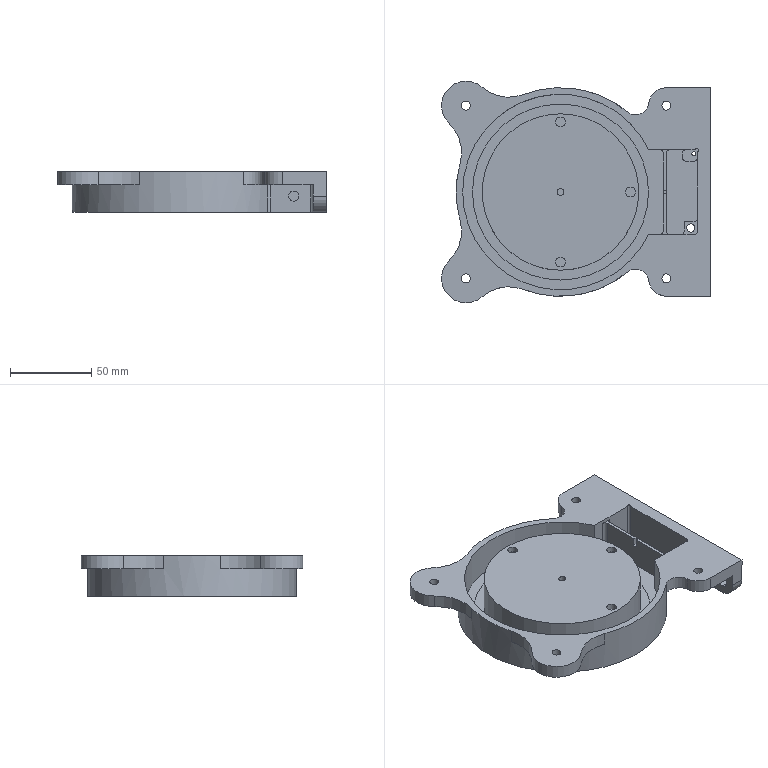NC program | NX | posted with a generic post | part box 165 x 136 x 25 mm
Lines 12614 to 13626 of 16615:
(CAVITY_MILL_COPY , TOOL : D4)
N25178 T04 M6
N25180 G54
N25182 G17 G0 G90 X-68.564 Y23.2 S9500 M3
N25184 G43 Z30. H4
N25186 Z0.602
N25188 G94 G1 Z-0.398 F1000.
N25190 X-68.737 Y23.5
N25192 G3 X-69.603 Y24. R1.
N25194 G1 X-72.5 F1500.
N25196 Y21.103
N25198 G3 X-72. Y20.237 R1.
N25200 G1 X-71.7 Y20.064
N25202 Z0.602
N25204 G0 Z30.
N25206 X-68.564 Y23.2
N25208 Z0.204
N25210 G1 Z-0.796 F1000.
N25212 X-68.737 Y23.5
N25214 G3 X-69.603 Y24. R1.
N25216 G1 X-72.5 F1500.
N25218 Y21.103
N25220 G3 X-72. Y20.237 R1.
N25222 G1 X-71.7 Y20.064
N25224 Z0.204
N25226 G0 X-68.564 Y23.2 Z-0.194
N25228 G1 Z-1.194 F1000.
N25230 X-68.737 Y23.5
N25232 G3 X-69.603 Y24. R1.
N25234 G1 X-72.5 F1500.
N25236 Y21.103
N25238 G3 X-72. Y20.237 R1.
N25240 G1 X-71.7 Y20.064
N25242 Z-0.194
N25244 G0 X-68.564 Y23.2 Z-0.592
N25246 G1 Z-1.592 F1000.
N25248 X-68.737 Y23.5
N25250 G3 X-69.603 Y24. R1.
N25252 G1 X-72.5 F1500.
N25254 Y21.103
N25256 G3 X-72. Y20.237 R1.
N25258 G1 X-71.7 Y20.064
N25260 Z-0.592
N25262 G0 X-68.564 Y23.2 Z-0.99
N25264 G1 Z-1.99 F1000.
N25266 X-68.737 Y23.5
N25268 G3 X-69.603 Y24. R1.
N25270 G1 X-72.5 F1500.
N25272 Y21.103
N25274 G3 X-72. Y20.237 R1.
N25276 G1 X-71.7 Y20.064
N25278 Z-0.99
N25280 G0 X-68.564 Y23.2 Z-1.388
N25282 G1 Z-2.388 F1000.
N25284 X-68.737 Y23.5
N25286 G3 X-69.603 Y24. R1.
N25288 G1 X-72.5 F1500.
N25290 Y21.103
N25292 G3 X-72. Y20.237 R1.
N25294 G1 X-71.7 Y20.064
N25296 Z-1.388
N25298 G0 X-68.564 Y23.2 Z-1.786
N25300 G1 Z-2.786 F1000.
N25302 X-68.737 Y23.5
N25304 G3 X-69.603 Y24. R1.
N25306 G1 X-72.5 F1500.
N25308 Y21.103
N25310 G3 X-72. Y20.237 R1.
N25312 G1 X-71.7 Y20.064
N25314 Z-1.786
N25316 G0 X-68.564 Y23.2 Z-2.184
N25318 G1 Z-3.184 F1000.
N25320 X-68.737 Y23.5
N25322 G3 X-69.603 Y24. R1.
N25324 G1 X-72.5 F1500.
N25326 Y21.103
N25328 G3 X-72. Y20.237 R1.
N25330 G1 X-71.7 Y20.064
N25332 Z-2.184
N25334 G0 X-68.564 Y23.2 Z-2.582
N25336 G1 Z-3.582 F1000.
N25338 X-68.737 Y23.5
N25340 G3 X-69.603 Y24. R1.
N25342 G1 X-72.5 F1500.
N25344 Y21.103
N25346 G3 X-72. Y20.237 R1.
N25348 G1 X-71.7 Y20.064
N25350 Z-2.582
N25352 G0 X-68.564 Y23.2 Z-2.98
N25354 G1 Z-3.98 F1000.
N25356 X-68.737 Y23.5
N25358 G3 X-69.603 Y24. R1.
N25360 G1 X-72.5 F1500.
N25362 Y21.103
N25364 G3 X-72. Y20.237 R1.
N25366 G1 X-71.7 Y20.064
N25368 Z-2.98
N25370 G0 X-68.564 Y23.2 Z-3.378
N25372 G1 Z-4.378 F1000.
N25374 X-68.737 Y23.5
N25376 G3 X-69.603 Y24. R1.
N25378 G1 X-72.5 F1500.
N25380 Y21.103
N25382 G3 X-72. Y20.237 R1.
N25384 G1 X-71.7 Y20.064
N25386 Z-3.378
N25388 G0 X-68.564 Y23.2 Z-3.776
N25390 G1 Z-4.776 F1000.
N25392 X-68.737 Y23.5
N25394 G3 X-69.603 Y24. R1.
N25396 G1 X-72.5 F1500.
N25398 Y21.103
N25400 G3 X-72. Y20.237 R1.
N25402 G1 X-71.7 Y20.064
N25404 Z-3.776
N25406 G0 X-68.564 Y23.2 Z-4.175
N25408 G1 Z-5.175 F1000.
N25410 X-68.737 Y23.5
N25412 G3 X-69.603 Y24. R1.
N25414 G1 X-72.5 F1500.
N25416 Y21.103
N25418 G3 X-72. Y20.237 R1.
N25420 G1 X-71.7 Y20.064
N25422 Z-4.175
N25424 G0 X-68.564 Y23.2 Z-4.573
N25426 G1 Z-5.573 F1000.
N25428 X-68.737 Y23.5
N25430 G3 X-69.603 Y24. R1.
N25432 G1 X-72.5 F1500.
N25434 Y21.103
N25436 G3 X-72. Y20.237 R1.
N25438 G1 X-71.7 Y20.064
N25440 Z-4.573
N25442 G0 X-68.564 Y23.2 Z-4.971
N25444 G1 Z-5.971 F1000.
N25446 X-68.737 Y23.5
N25448 G3 X-69.603 Y24. R1.
N25450 G1 X-72.5 F1500.
N25452 Y21.103
N25454 G3 X-72. Y20.237 R1.
N25456 G1 X-71.7 Y20.064
N25458 Z-4.971
N25460 G0 X-68.564 Y23.2 Z-5.369
N25462 G1 Z-6.369 F1000.
N25464 X-68.737 Y23.5
N25466 G3 X-69.603 Y24. R1.
N25468 G1 X-72.5 F1500.
N25470 Y21.103
N25472 G3 X-72. Y20.237 R1.
N25474 G1 X-71.7 Y20.064
N25476 Z-5.369
N25478 G0 X-68.564 Y23.2 Z-5.767
N25480 G1 Z-6.767 F1000.
N25482 X-68.737 Y23.5
N25484 G3 X-69.603 Y24. R1.
N25486 G1 X-72.5 F1500.
N25488 Y21.103
N25490 G3 X-72. Y20.237 R1.
N25492 G1 X-71.7 Y20.064
N25494 Z-5.767
N25496 G0 X-68.564 Y23.2 Z-6.165
N25498 G1 Z-7.165 F1000.
N25500 X-68.737 Y23.5
N25502 G3 X-69.603 Y24. R1.
N25504 G1 X-72.5 F1500.
N25506 Y21.103
N25508 G3 X-72. Y20.237 R1.
N25510 G1 X-71.7 Y20.064
N25512 Z-6.165
N25514 G0 X-68.564 Y23.2 Z-6.563
N25516 G1 Z-7.563 F1000.
N25518 X-68.737 Y23.5
N25520 G3 X-69.603 Y24. R1.
N25522 G1 X-72.5 F1500.
N25524 Y21.103
N25526 G3 X-72. Y20.237 R1.
N25528 G1 X-71.7 Y20.064
N25530 Z-6.563
N25532 G0 X-68.564 Y23.2 Z-6.961
N25534 G1 Z-7.961 F1000.
N25536 X-68.737 Y23.5
N25538 G3 X-69.603 Y24. R1.
N25540 G1 X-72.5 F1500.
N25542 Y21.103
N25544 G3 X-72. Y20.237 R1.
N25546 G1 X-71.7 Y20.064
N25548 Z-6.961
N25550 G0 X-68.564 Y23.2 Z-7.359
N25552 G1 Z-8.359 F1000.
N25554 X-68.737 Y23.5
N25556 G3 X-69.603 Y24. R1.
N25558 G1 X-72.5 F1500.
N25560 Y21.103
N25562 G3 X-72. Y20.237 R1.
N25564 G1 X-71.7 Y20.064
N25566 Z-7.359
N25568 G0 X-68.564 Y23.2 Z-7.757
N25570 G1 Z-8.757 F1000.
N25572 X-68.737 Y23.5
N25574 G3 X-69.603 Y24. R1.
N25576 G1 X-72.5 F1500.
N25578 Y21.103
N25580 G3 X-72. Y20.237 R1.
N25582 G1 X-71.7 Y20.064
N25584 Z-7.757
N25586 G0 X-68.564 Y23.2 Z-8.155
N25588 G1 Z-9.155 F1000.
N25590 X-68.737 Y23.5
N25592 G3 X-69.603 Y24. R1.
N25594 G1 X-72.5 F1500.
N25596 Y21.103
N25598 G3 X-72. Y20.237 R1.
N25600 G1 X-71.7 Y20.064
N25602 Z-8.155
N25604 G0 X-68.564 Y23.2 Z-8.553
N25606 G1 Z-9.553 F1000.
N25608 X-68.737 Y23.5
N25610 G3 X-69.603 Y24. R1.
N25612 G1 X-72.5 F1500.
N25614 Y21.103
N25616 G3 X-72. Y20.237 R1.
N25618 G1 X-71.7 Y20.064
N25620 Z-8.553
N25622 G0 X-68.564 Y23.2 Z-8.951
N25624 G1 Z-9.951 F1000.
N25626 X-68.737 Y23.5
N25628 G3 X-69.603 Y24. R1.
N25630 G1 X-72.5 F1500.
N25632 Y21.103
N25634 G3 X-72. Y20.237 R1.
N25636 G1 X-71.7 Y20.064
N25638 Z-8.951
N25640 G0 X-68.564 Y23.2 Z-9.349
N25642 G1 Z-10.349 F1000.
N25644 X-68.737 Y23.5
N25646 G3 X-69.603 Y24. R1.
N25648 G1 X-72.5 F1500.
N25650 Y21.103
N25652 G3 X-72. Y20.237 R1.
N25654 G1 X-71.7 Y20.064
N25656 Z-9.349
N25658 G0 X-68.564 Y23.2 Z-9.747
N25660 G1 Z-10.747 F1000.
N25662 X-68.737 Y23.5
N25664 G3 X-69.603 Y24. R1.
N25666 G1 X-72.5 F1500.
N25668 Y21.103
N25670 G3 X-72. Y20.237 R1.
N25672 G1 X-71.7 Y20.064
N25674 Z-9.747
N25676 G0 X-68.564 Y23.2 Z-10.145
N25678 G1 Z-11.145 F1000.
N25680 X-68.737 Y23.5
N25682 G3 X-69.603 Y24. R1.
N25684 G1 X-72.5 F1500.
N25686 Y21.103
N25688 G3 X-72. Y20.237 R1.
N25690 G1 X-71.7 Y20.064
N25692 Z-10.145
N25694 G0 X-68.564 Y23.2 Z-10.543
N25696 G1 Z-11.543 F1000.
N25698 X-68.737 Y23.5
N25700 G3 X-69.603 Y24. R1.
N25702 G1 X-72.5 F1500.
N25704 Y21.103
N25706 G3 X-72. Y20.237 R1.
N25708 G1 X-71.7 Y20.064
N25710 Z-10.543
N25712 G0 X-68.564 Y23.2 Z-10.941
N25714 G1 Z-11.941 F1000.
N25716 X-68.737 Y23.5
N25718 G3 X-69.603 Y24. R1.
N25720 G1 X-72.5 F1500.
N25722 Y21.103
N25724 G3 X-72. Y20.237 R1.
N25726 G1 X-71.7 Y20.064
N25728 Z-10.941
N25730 G0 X-68.564 Y23.2 Z-11.339
N25732 G1 Z-12.339 F1000.
N25734 X-68.737 Y23.5
N25736 G3 X-69.603 Y24. R1.
N25738 G1 X-72.5 F1500.
N25740 Y21.103
N25742 G3 X-72. Y20.237 R1.
N25744 G1 X-71.7 Y20.064
N25746 Z-11.339
N25748 G0 X-68.564 Y23.2 Z-11.737
N25750 G1 Z-12.737 F1000.
N25752 X-68.737 Y23.5
N25754 G3 X-69.603 Y24. R1.
N25756 G1 X-72.5 F1500.
N25758 Y21.103
N25760 G3 X-72. Y20.237 R1.
N25762 G1 X-71.7 Y20.064
N25764 Z-11.737
N25766 G0 X-68.564 Y23.2 Z-12.135
N25768 G1 Z-13.135 F1000.
N25770 X-68.737 Y23.5
N25772 G3 X-69.603 Y24. R1.
N25774 G1 X-72.5 F1500.
N25776 Y21.103
N25778 G3 X-72. Y20.237 R1.
N25780 G1 X-71.7 Y20.064
N25782 Z-12.135
N25784 G0 X-68.564 Y23.2 Z-12.533
N25786 G1 Z-13.533 F1000.
N25788 X-68.737 Y23.5
N25790 G3 X-69.603 Y24. R1.
N25792 G1 X-72.5 F1500.
N25794 Y21.103
N25796 G3 X-72. Y20.237 R1.
N25798 G1 X-71.7 Y20.064
N25800 Z-12.533
N25802 G0 X-68.564 Y23.2 Z-12.931
N25804 G1 Z-13.931 F1000.
N25806 X-68.737 Y23.5
N25808 G3 X-69.603 Y24. R1.
N25810 G1 X-72.5 F1500.
N25812 Y21.103
N25814 G3 X-72. Y20.237 R1.
N25816 G1 X-71.7 Y20.064
N25818 Z-12.931
N25820 G0 X-68.564 Y23.2 Z-13.329
N25822 G1 Z-14.329 F1000.
N25824 X-68.737 Y23.5
N25826 G3 X-69.603 Y24. R1.
N25828 G1 X-72.5 F1500.
N25830 Y21.103
N25832 G3 X-72. Y20.237 R1.
N25834 G1 X-71.7 Y20.064
N25836 Z-13.329
N25838 G0 X-68.564 Y23.2 Z-13.727
N25840 G1 Z-14.727 F1000.
N25842 X-68.737 Y23.5
N25844 G3 X-69.603 Y24. R1.
N25846 G1 X-72.5 F1500.
N25848 Y21.103
N25850 G3 X-72. Y20.237 R1.
N25852 G1 X-71.7 Y20.064
N25854 Z-13.727
N25856 G0 X-68.564 Y23.2 Z-14.125
N25858 G1 Z-15.125 F1000.
N25860 X-68.737 Y23.5
N25862 G3 X-69.603 Y24. R1.
N25864 G1 X-72.5 F1500.
N25866 Y21.103
N25868 G3 X-72. Y20.237 R1.
N25870 G1 X-71.7 Y20.064
N25872 Z-14.125
N25874 G0 X-68.564 Y23.2 Z-14.524
N25876 G1 Z-15.524 F1000.
N25878 X-68.737 Y23.5
N25880 G3 X-69.603 Y24. R1.
N25882 G1 X-72.5 F1500.
N25884 Y21.103
N25886 G3 X-72. Y20.237 R1.
N25888 G1 X-71.7 Y20.064
N25890 Z-14.524
N25892 G0 X-68.564 Y23.2 Z-14.922
N25894 G1 Z-15.922 F1000.
N25896 X-68.737 Y23.5
N25898 G3 X-69.603 Y24. R1.
N25900 G1 X-72.5 F1500.
N25902 Y21.103
N25904 G3 X-72. Y20.237 R1.
N25906 G1 X-71.7 Y20.064
N25908 Z-14.922
N25910 G0 X-68.564 Y23.2 Z-15.32
N25912 G1 Z-16.32 F1000.
N25914 X-68.737 Y23.5
N25916 G3 X-69.603 Y24. R1.
N25918 G1 X-72.5 F1500.
N25920 Y21.103
N25922 G3 X-72. Y20.237 R1.
N25924 G1 X-71.7 Y20.064
N25926 Z-15.32
N25928 G0 X-68.564 Y23.2 Z-15.718
N25930 G1 Z-16.718 F1000.
N25932 X-68.737 Y23.5
N25934 G3 X-69.603 Y24. R1.
N25936 G1 X-72.5 F1500.
N25938 Y21.103
N25940 G3 X-72. Y20.237 R1.
N25942 G1 X-71.7 Y20.064
N25944 Z-15.718
N25946 G0 X-68.564 Y23.2 Z-16.116
N25948 G1 Z-17.116 F1000.
N25950 X-68.737 Y23.5
N25952 G3 X-69.603 Y24. R1.
N25954 G1 X-72.5 F1500.
N25956 Y21.103
N25958 G3 X-72. Y20.237 R1.
N25960 G1 X-71.7 Y20.064
N25962 Z-16.116
N25964 G0 X-68.564 Y23.2 Z-16.514
N25966 G1 Z-17.514 F1000.
N25968 X-68.737 Y23.5
N25970 G3 X-69.603 Y24. R1.
N25972 G1 X-72.5 F1500.
N25974 Y21.103
N25976 G3 X-72. Y20.237 R1.
N25978 G1 X-71.7 Y20.064
N25980 Z-16.514
N25982 G0 X-68.564 Y23.2 Z-16.912
N25984 G1 Z-17.912 F1000.
N25986 X-68.737 Y23.5
N25988 G3 X-69.603 Y24. R1.
N25990 G1 X-72.5 F1500.
N25992 Y21.103
N25994 G3 X-72. Y20.237 R1.
N25996 G1 X-71.7 Y20.064
N25998 Z-16.912
N26000 G0 X-68.564 Y23.2 Z-17.31
N26002 G1 Z-18.31 F1000.
N26004 X-68.737 Y23.5
N26006 G3 X-69.603 Y24. R1.
N26008 G1 X-72.5 F1500.
N26010 Y21.103
N26012 G3 X-72. Y20.237 R1.
N26014 G1 X-71.7 Y20.064
N26016 Z-17.31
N26018 G0 X-68.564 Y23.2 Z-17.708
N26020 G1 Z-18.708 F1000.
N26022 X-68.737 Y23.5
N26024 G3 X-69.603 Y24. R1.
N26026 G1 X-72.5 F1500.
N26028 Y21.103
N26030 G3 X-72. Y20.237 R1.
N26032 G1 X-71.7 Y20.064
N26034 Z-17.708
N26036 G0 X-68.564 Y23.2 Z-18.106
N26038 G1 Z-19.106 F1000.
N26040 X-68.737 Y23.5
N26042 G3 X-69.603 Y24. R1.
N26044 G1 X-72.5 F1500.
N26046 Y21.103
N26048 G3 X-72. Y20.237 R1.
N26050 G1 X-71.7 Y20.064
N26052 Z-18.106
N26054 G0 X-68.564 Y23.2 Z-18.504
N26056 G1 Z-19.504 F1000.
N26058 X-68.737 Y23.5
N26060 G3 X-69.603 Y24. R1.
N26062 G1 X-72.5 F1500.
N26064 Y21.103
N26066 G3 X-72. Y20.237 R1.
N26068 G1 X-71.7 Y20.064
N26070 Z-18.504
N26072 G0 X-68.564 Y23.2 Z-18.902
N26074 G1 Z-19.902 F1000.
N26076 X-68.737 Y23.5
N26078 G3 X-69.603 Y24. R1.
N26080 G1 X-72.5 F1500.
N26082 Y21.103
N26084 G3 X-72. Y20.237 R1.
N26086 G1 X-71.7 Y20.064
N26088 Z-18.902
N26090 G0 X-68.564 Y23.2 Z-19.3
N26092 G1 Z-20.3 F1000.
N26094 X-68.737 Y23.5
N26096 G3 X-69.603 Y24. R1.
N26098 G1 X-72.5 F1500.
N26100 Y21.103
N26102 G3 X-72. Y20.237 R1.
N26104 G1 X-71.7 Y20.064
N26106 Z-19.3
N26108 G0 Z30.
N26110 X-68.564 Y15.2
N26112 Z-19.65
N26114 G1 Z-20.65 F1000.
N26116 X-68.737 Y15.5
N26118 G3 X-69.603 Y16. R1.
N26120 G1 X-72.5 F1500.
N26122 Y13.103
N26124 G3 X-72. Y12.237 R1.
N26126 G1 X-71.7 Y12.064
N26128 Z-19.65
N26130 G0 X-68.564 Y15.2 Z-20.
N26132 G1 Z-21. F1000.
N26134 X-68.737 Y15.5
N26136 G3 X-69.603 Y16. R1.
N26138 G1 X-72.5 F1500.
N26140 Y13.103
N26142 G3 X-72. Y12.237 R1.
N26144 G1 X-71.7 Y12.064
N26146 Z-20.
N26148 G0 Z30.
N26150 X-58.3 Y20.064
N26152 Z-1.388
N26154 G1 Z-2.388 F1000.
N26156 X-58. Y20.237
N26158 G3 X-57.5 Y21.103 R1.
N26160 G1 Y24. F1500.
N26162 X-60.397
N26164 G3 X-61.263 Y23.5 R1.
N26166 G1 X-61.436 Y23.2
N26168 Z-1.388
N26170 G0 X-58.3 Y20.064 Z-1.786
N26172 G1 Z-2.786 F1000.
N26174 X-58. Y20.237
N26176 G3 X-57.5 Y21.103 R1.
N26178 G1 Y24. F1500.
N26180 X-60.397
N26182 G3 X-61.263 Y23.5 R1.
N26184 G1 X-61.436 Y23.2
N26186 Z-1.786
N26188 G0 X-58.3 Y20.064 Z-2.184
N26190 G1 Z-3.184 F1000.
N26192 X-58. Y20.237
N26194 G3 X-57.5 Y21.103 R1.
N26196 G1 Y24. F1500.
N26198 X-60.397
N26200 G3 X-61.263 Y23.5 R1.
N26202 G1 X-61.436 Y23.2
N26204 Z-2.184
N26206 G0 X-58.3 Y20.064 Z-2.582
N26208 G1 Z-3.582 F1000.
N26210 X-58. Y20.237
N26212 G3 X-57.5 Y21.103 R1.
N26214 G1 Y24. F1500.
N26216 X-60.397
N26218 G3 X-61.263 Y23.5 R1.
N26220 G1 X-61.436 Y23.2
N26222 Z-2.582
N26224 G0 X-58.3 Y20.064 Z-2.98
N26226 G1 Z-3.98 F1000.
N26228 X-58. Y20.237
N26230 G3 X-57.5 Y21.103 R1.
N26232 G1 Y24. F1500.
N26234 X-60.397
N26236 G3 X-61.263 Y23.5 R1.
N26238 G1 X-61.436 Y23.2
N26240 Z-2.98
N26242 G0 X-58.3 Y20.064 Z-3.378
N26244 G1 Z-4.378 F1000.
N26246 X-58. Y20.237
N26248 G3 X-57.5 Y21.103 R1.
N26250 G1 Y24. F1500.
N26252 X-60.397
N26254 G3 X-61.263 Y23.5 R1.
N26256 G1 X-61.436 Y23.2
N26258 Z-3.378
N26260 G0 X-58.3 Y20.064 Z-3.776
N26262 G1 Z-4.776 F1000.
N26264 X-58. Y20.237
N26266 G3 X-57.5 Y21.103 R1.
N26268 G1 Y24. F1500.
N26270 X-60.397
N26272 G3 X-61.263 Y23.5 R1.
N26274 G1 X-61.436 Y23.2
N26276 Z-3.776
N26278 G0 X-58.3 Y20.064 Z-4.175
N26280 G1 Z-5.175 F1000.
N26282 X-58. Y20.237
N26284 G3 X-57.5 Y21.103 R1.
N26286 G1 Y24. F1500.
N26288 X-60.397
N26290 G3 X-61.263 Y23.5 R1.
N26292 G1 X-61.436 Y23.2
N26294 Z-4.175
N26296 G0 X-58.3 Y20.064 Z-4.573
N26298 G1 Z-5.573 F1000.
N26300 X-58. Y20.237
N26302 G3 X-57.5 Y21.103 R1.
N26304 G1 Y24. F1500.
N26306 X-60.397
N26308 G3 X-61.263 Y23.5 R1.
N26310 G1 X-61.436 Y23.2
N26312 Z-4.573
N26314 G0 X-58.3 Y20.064 Z-4.971
N26316 G1 Z-5.971 F1000.
N26318 X-58. Y20.237
N26320 G3 X-57.5 Y21.103 R1.
N26322 G1 Y24. F1500.
N26324 X-60.397
N26326 G3 X-61.263 Y23.5 R1.
N26328 G1 X-61.436 Y23.2
N26330 Z-4.971
N26332 G0 X-58.3 Y20.064 Z-5.369
N26334 G1 Z-6.369 F1000.
N26336 X-58. Y20.237
N26338 G3 X-57.5 Y21.103 R1.
N26340 G1 Y24. F1500.
N26342 X-60.397
N26344 G3 X-61.263 Y23.5 R1.
N26346 G1 X-61.436 Y23.2
N26348 Z-5.369
N26350 G0 X-58.3 Y20.064 Z-5.767
N26352 G1 Z-6.767 F1000.
N26354 X-58. Y20.237
N26356 G3 X-57.5 Y21.103 R1.
N26358 G1 Y24. F1500.
N26360 X-60.397
N26362 G3 X-61.263 Y23.5 R1.
N26364 G1 X-61.436 Y23.2
N26366 Z-5.767
N26368 G0 X-58.3 Y20.064 Z-6.165
N26370 G1 Z-7.165 F1000.
N26372 X-58. Y20.237
N26374 G3 X-57.5 Y21.103 R1.
N26376 G1 Y24. F1500.
N26378 X-60.397
N26380 G3 X-61.263 Y23.5 R1.
N26382 G1 X-61.436 Y23.2
N26384 Z-6.165
N26386 G0 X-58.3 Y20.064 Z-6.563
N26388 G1 Z-7.563 F1000.
N26390 X-58. Y20.237
N26392 G3 X-57.5 Y21.103 R1.
N26394 G1 Y24. F1500.
N26396 X-60.397
N26398 G3 X-61.263 Y23.5 R1.
N26400 G1 X-61.436 Y23.2
N26402 Z-6.563
N26404 G0 X-58.3 Y20.064 Z-6.961
N26406 G1 Z-7.961 F1000.
N26408 X-58. Y20.237
N26410 G3 X-57.5 Y21.103 R1.
N26412 G1 Y24. F1500.
N26414 X-60.397
N26416 G3 X-61.263 Y23.5 R1.
N26418 G1 X-61.436 Y23.2
N26420 Z-6.961
N26422 G0 X-58.3 Y20.064 Z-7.359
N26424 G1 Z-8.359 F1000.
N26426 X-58. Y20.237
N26428 G3 X-57.5 Y21.103 R1.
N26430 G1 Y24. F1500.
N26432 X-60.397
N26434 G3 X-61.263 Y23.5 R1.
N26436 G1 X-61.436 Y23.2
N26438 Z-7.359
N26440 G0 X-58.3 Y20.064 Z-7.757
N26442 G1 Z-8.757 F1000.
N26444 X-58. Y20.237
N26446 G3 X-57.5 Y21.103 R1.
N26448 G1 Y24. F1500.
N26450 X-60.397
N26452 G3 X-61.263 Y23.5 R1.
N26454 G1 X-61.436 Y23.2
N26456 Z-7.757
N26458 G0 X-58.3 Y20.064 Z-8.155
N26460 G1 Z-9.155 F1000.
N26462 X-58. Y20.237
N26464 G3 X-57.5 Y21.103 R1.
N26466 G1 Y24. F1500.
N26468 X-60.397
N26470 G3 X-61.263 Y23.5 R1.
N26472 G1 X-61.436 Y23.2
N26474 Z-8.155
N26476 G0 X-58.3 Y20.064 Z-8.553
N26478 G1 Z-9.553 F1000.
N26480 X-58. Y20.237
N26482 G3 X-57.5 Y21.103 R1.
N26484 G1 Y24. F1500.
N26486 X-60.397
N26488 G3 X-61.263 Y23.5 R1.
N26490 G1 X-61.436 Y23.2
N26492 Z-8.553
N26494 G0 X-58.3 Y20.064 Z-8.951
N26496 G1 Z-9.951 F1000.
N26498 X-58. Y20.237
N26500 G3 X-57.5 Y21.103 R1.
N26502 G1 Y24. F1500.
N26504 X-60.397
N26506 G3 X-61.263 Y23.5 R1.
N26508 G1 X-61.436 Y23.2
N26510 Z-8.951
N26512 G0 X-58.3 Y20.064 Z-9.349
N26514 G1 Z-10.349 F1000.
N26516 X-58. Y20.237
N26518 G3 X-57.5 Y21.103 R1.
N26520 G1 Y24. F1500.
N26522 X-60.397
N26524 G3 X-61.263 Y23.5 R1.
N26526 G1 X-61.436 Y23.2
N26528 Z-9.349
N26530 G0 X-58.3 Y20.064 Z-9.747
N26532 G1 Z-10.747 F1000.
N26534 X-58. Y20.237
N26536 G3 X-57.5 Y21.103 R1.
N26538 G1 Y24. F1500.
N26540 X-60.397
N26542 G3 X-61.263 Y23.5 R1.
N26544 G1 X-61.436 Y23.2
N26546 Z-9.747
N26548 G0 X-58.3 Y20.064 Z-10.145
N26550 G1 Z-11.145 F1000.
N26552 X-58. Y20.237
N26554 G3 X-57.5 Y21.103 R1.
N26556 G1 Y24. F1500.
N26558 X-60.397
N26560 G3 X-61.263 Y23.5 R1.
N26562 G1 X-61.436 Y23.2
N26564 Z-10.145
N26566 G0 X-58.3 Y20.064 Z-10.543
N26568 G1 Z-11.543 F1000.
N26570 X-58. Y20.237
N26572 G3 X-57.5 Y21.103 R1.
N26574 G1 Y24. F1500.
N26576 X-60.397
N26578 G3 X-61.263 Y23.5 R1.
N26580 G1 X-61.436 Y23.2
N26582 Z-10.543
N26584 G0 X-58.3 Y20.064 Z-10.941
N26586 G1 Z-11.941 F1000.
N26588 X-58. Y20.237
N26590 G3 X-57.5 Y21.103 R1.
N26592 G1 Y24. F1500.
N26594 X-60.397
N26596 G3 X-61.263 Y23.5 R1.
N26598 G1 X-61.436 Y23.2
N26600 Z-10.941
N26602 G0 X-58.3 Y20.064 Z-11.339
N26604 G1 Z-12.339 F1000.
N26606 X-58. Y20.237
N26608 G3 X-57.5 Y21.103 R1.
N26610 G1 Y24. F1500.
N26612 X-60.397
N26614 G3 X-61.263 Y23.5 R1.
N26616 G1 X-61.436 Y23.2
N26618 Z-11.339
N26620 G0 X-58.3 Y20.064 Z-11.737
N26622 G1 Z-12.737 F1000.
N26624 X-58. Y20.237
N26626 G3 X-57.5 Y21.103 R1.
N26628 G1 Y24. F1500.
N26630 X-60.397
N26632 G3 X-61.263 Y23.5 R1.
N26634 G1 X-61.436 Y23.2
N26636 Z-11.737
N26638 G0 X-58.3 Y20.064 Z-12.135
N26640 G1 Z-13.135 F1000.
N26642 X-58. Y20.237
N26644 G3 X-57.5 Y21.103 R1.
N26646 G1 Y24. F1500.
N26648 X-60.397
N26650 G3 X-61.263 Y23.5 R1.
N26652 G1 X-61.436 Y23.2
N26654 Z-12.135
N26656 G0 X-58.3 Y20.064 Z-12.533
N26658 G1 Z-13.533 F1000.
N26660 X-58. Y20.237
N26662 G3 X-57.5 Y21.103 R1.
N26664 G1 Y24. F1500.
N26666 X-60.397
N26668 G3 X-61.263 Y23.5 R1.
N26670 G1 X-61.436 Y23.2
N26672 Z-12.533
N26674 G0 X-58.3 Y20.064 Z-12.931
N26676 G1 Z-13.931 F1000.
N26678 X-58. Y20.237
N26680 G3 X-57.5 Y21.103 R1.
N26682 G1 Y24. F1500.
N26684 X-60.397
N26686 G3 X-61.263 Y23.5 R1.
N26688 G1 X-61.436 Y23.2
N26690 Z-12.931
N26692 G0 X-58.3 Y20.064 Z-13.329
N26694 G1 Z-14.329 F1000.
N26696 X-58. Y20.237
N26698 G3 X-57.5 Y21.103 R1.
N26700 G1 Y24. F1500.
N26702 X-60.397
N26704 G3 X-61.263 Y23.5 R1.
N26706 G1 X-61.436 Y23.2
N26708 Z-13.329
N26710 G0 X-58.3 Y20.064 Z-13.727
N26712 G1 Z-14.727 F1000.
N26714 X-58. Y20.237
N26716 G3 X-57.5 Y21.103 R1.
N26718 G1 Y24. F1500.
N26720 X-60.397
N26722 G3 X-61.263 Y23.5 R1.
N26724 G1 X-61.436 Y23.2
N26726 Z-13.727
N26728 G0 X-58.3 Y20.064 Z-14.125
N26730 G1 Z-15.125 F1000.
N26732 X-58. Y20.237
N26734 G3 X-57.5 Y21.103 R1.
N26736 G1 Y24. F1500.
N26738 X-60.397
N26740 G3 X-61.263 Y23.5 R1.
N26742 G1 X-61.436 Y23.2
N26744 Z-14.125
N26746 G0 X-58.3 Y20.064 Z-14.524
N26748 G1 Z-15.524 F1000.
N26750 X-58. Y20.237
N26752 G3 X-57.5 Y21.103 R1.
N26754 G1 Y24. F1500.
N26756 X-60.397
N26758 G3 X-61.263 Y23.5 R1.
N26760 G1 X-61.436 Y23.2
N26762 Z-14.524
N26764 G0 X-58.3 Y20.064 Z-14.922
N26766 G1 Z-15.922 F1000.
N26768 X-58. Y20.237
N26770 G3 X-57.5 Y21.103 R1.
N26772 G1 Y24. F1500.
N26774 X-60.397
N26776 G3 X-61.263 Y23.5 R1.
N26778 G1 X-61.436 Y23.2
N26780 Z-14.922
N26782 G0 X-58.3 Y20.064 Z-15.32
N26784 G1 Z-16.32 F1000.
N26786 X-58. Y20.237
N26788 G3 X-57.5 Y21.103 R1.
N26790 G1 Y24. F1500.
N26792 X-60.397
N26794 G3 X-61.263 Y23.5 R1.
N26796 G1 X-61.436 Y23.2
N26798 Z-15.32
N26800 G0 X-58.3 Y20.064 Z-15.718
N26802 G1 Z-16.718 F1000.
N26804 X-58. Y20.237
N26806 G3 X-57.5 Y21.103 R1.
N26808 G1 Y24. F1500.
N26810 X-60.397
N26812 G3 X-61.263 Y23.5 R1.
N26814 G1 X-61.436 Y23.2
N26816 Z-15.718
N26818 G0 X-58.3 Y20.064 Z-16.116
N26820 G1 Z-17.116 F1000.
N26822 X-58. Y20.237
N26824 G3 X-57.5 Y21.103 R1.
N26826 G1 Y24. F1500.
N26828 X-60.397
N26830 G3 X-61.263 Y23.5 R1.
N26832 G1 X-61.436 Y23.2
N26834 Z-16.116
N26836 G0 X-58.3 Y20.064 Z-16.514
N26838 G1 Z-17.514 F1000.
N26840 X-58. Y20.237
N26842 G3 X-57.5 Y21.103 R1.
N26844 G1 Y24. F1500.
N26846 X-60.397
N26848 G3 X-61.263 Y23.5 R1.
N26850 G1 X-61.436 Y23.2
N26852 Z-16.514
N26854 G0 X-58.3 Y20.064 Z-16.912
N26856 G1 Z-17.912 F1000.
N26858 X-58. Y20.237
N26860 G3 X-57.5 Y21.103 R1.
N26862 G1 Y24. F1500.
N26864 X-60.397
N26866 G3 X-61.263 Y23.5 R1.
N26868 G1 X-61.436 Y23.2
N26870 Z-16.912
N26872 G0 X-58.3 Y20.064 Z-17.31
N26874 G1 Z-18.31 F1000.
N26876 X-58. Y20.237
N26878 G3 X-57.5 Y21.103 R1.
N26880 G1 Y24. F1500.
N26882 X-60.397
N26884 G3 X-61.263 Y23.5 R1.
N26886 G1 X-61.436 Y23.2
N26888 Z-17.31
N26890 G0 X-58.3 Y20.064 Z-17.708
N26892 G1 Z-18.708 F1000.
N26894 X-58. Y20.237
N26896 G3 X-57.5 Y21.103 R1.
N26898 G1 Y24. F1500.
N26900 X-60.397
N26902 G3 X-61.263 Y23.5 R1.
N26904 G1 X-61.436 Y23.2
N26906 Z-17.708
N26908 G0 X-58.3 Y20.064 Z-18.106
N26910 G1 Z-19.106 F1000.
N26912 X-58. Y20.237
N26914 G3 X-57.5 Y21.103 R1.
N26916 G1 Y24. F1500.
N26918 X-60.397
N26920 G3 X-61.263 Y23.5 R1.
N26922 G1 X-61.436 Y23.2
N26924 Z-18.106
N26926 G0 X-58.3 Y20.064 Z-18.504
N26928 G1 Z-19.504 F1000.
N26930 X-58. Y20.237
N26932 G3 X-57.5 Y21.103 R1.
N26934 G1 Y24. F1500.
N26936 X-60.397
N26938 G3 X-61.263 Y23.5 R1.
N26940 G1 X-61.436 Y23.2
N26942 Z-18.504
N26944 G0 X-58.3 Y20.064 Z-18.902
N26946 G1 Z-19.902 F1000.
N26948 X-58. Y20.237
N26950 G3 X-57.5 Y21.103 R1.
N26952 G1 Y24. F1500.
N26954 X-60.397
N26956 G3 X-61.263 Y23.5 R1.
N26958 G1 X-61.436 Y23.2
N26960 Z-18.902
N26962 G0 X-58.3 Y20.064 Z-19.3
N26964 G1 Z-20.3 F1000.
N26966 X-58. Y20.237
N26968 G3 X-57.5 Y21.103 R1.
N26970 G1 Y24. F1500.
N26972 X-60.397
N26974 G3 X-61.263 Y23.5 R1.
N26976 G1 X-61.436 Y23.2
N26978 Z-19.3
N26980 G0 X-60.564 Z-19.65
N26982 G1 Z-20.65 F1000.
N26984 X-60.737 Y23.5
N26986 G3 X-61.603 Y24. R1.
N26988 G1 X-64.5 F1500.
N26990 Y21.103
N26992 G3 X-64. Y20.237 R1.
N26994 G1 X-63.7 Y20.064
N26996 Z-19.65
N26998 G0 X-60.564 Y23.2 Z-20.
N27000 G1 Z-21. F1000.
N27002 X-60.737 Y23.5
N27004 G3 X-61.603 Y24. R1.
N27006 G1 X-64.5 F1500.
N27008 Y21.103
N27010 G3 X-64. Y20.237 R1.
N27012 G1 X-63.7 Y20.064
N27014 Z-20.
N27016 G0 Z30.
N27018 X-58.3
N27020 Z-19.65
N27022 G1 Z-20.65 F1000.
N27024 X-58. Y20.237
N27026 G3 X-57.5 Y21.103 R1.
N27028 G1 Y24. F1500.
N27030 X-60.397
N27032 G3 X-61.263 Y23.5 R1.
N27034 G1 X-61.436 Y23.2
N27036 Z-19.65
N27038 G0 X-58.3 Y20.064 Z-20.
N27040 G1 Z-21. F1000.
N27042 X-58. Y20.237
N27044 G3 X-57.5 Y21.103 R1.
N27046 G1 Y24. F1500.
N27048 X-60.397
N27050 G3 X-61.263 Y23.5 R1.
N27052 G1 X-61.436 Y23.2
N27054 Z-20.
N27056 G0 Z30.
N27058 X-49.462 Y20.804
N27060 Z-1.388
N27062 G1 Z-2.388 F1000.
N27064 X-50.939 Y21.657
N27066 G2 X-51.439 Y22.523 R1.
N27068 G1 Y23.939 F1500.
N27070 X-48.607
N27072 X-48.603 Y24.
N27074 X-51.5
N27076 Y21.103
N27078 X-51.439 Y21.107
N27080 Y22.523
N27082 G2 X-50.939 Y23.389 R1.
N27084 G1 X-49.439 Y21.939
N27086 Z-1.388
N27088 G0 X-49.462 Y20.804 Z-1.786
N27090 G1 Z-2.786 F1000.
N27092 X-50.939 Y21.657
N27094 G2 X-51.439 Y22.523 R1.
N27096 G1 Y23.939 F1500.
N27098 X-48.607
N27100 X-48.603 Y24.
N27102 X-51.5
N27104 Y21.103
N27106 X-51.439 Y21.107
N27108 Y22.523
N27110 G2 X-50.939 Y23.389 R1.
N27112 G1 X-49.439 Y21.939
N27114 Z-1.786
N27116 G0 X-49.462 Y20.804 Z-2.184
N27118 G1 Z-3.184 F1000.
N27120 X-50.939 Y21.657
N27122 G2 X-51.439 Y22.523 R1.
N27124 G1 Y23.939 F1500.
N27126 X-48.607
N27128 X-48.603 Y24.
N27130 X-51.5
N27132 Y21.103
N27134 X-51.439 Y21.107
N27136 Y22.523
N27138 G2 X-50.939 Y23.389 R1.
N27140 G1 X-49.439 Y21.939
N27142 Z-2.184
N27144 G0 X-49.462 Y20.804 Z-2.582
N27146 G1 Z-3.582 F1000.
N27148 X-50.939 Y21.657
N27150 G2 X-51.439 Y22.523 R1.
N27152 G1 Y23.939 F1500.
N27154 X-48.607
N27156 X-48.603 Y24.
N27158 X-51.5
N27160 Y21.103
N27162 X-51.439 Y21.107
N27164 Y22.523
N27166 G2 X-50.939 Y23.389 R1.
N27168 G1 X-49.439 Y21.939
N27170 Z-2.582
N27172 G0 X-49.462 Y20.804 Z-2.98
N27174 G1 Z-3.98 F1000.
N27176 X-50.939 Y21.657
N27178 G2 X-51.439 Y22.523 R1.
N27180 G1 Y23.939 F1500.
N27182 X-48.607
N27184 X-48.603 Y24.
N27186 X-51.5
N27188 Y21.103
N27190 X-51.439 Y21.107
N27192 Y22.523
N27194 G2 X-50.939 Y23.389 R1.
N27196 G1 X-49.439 Y21.939